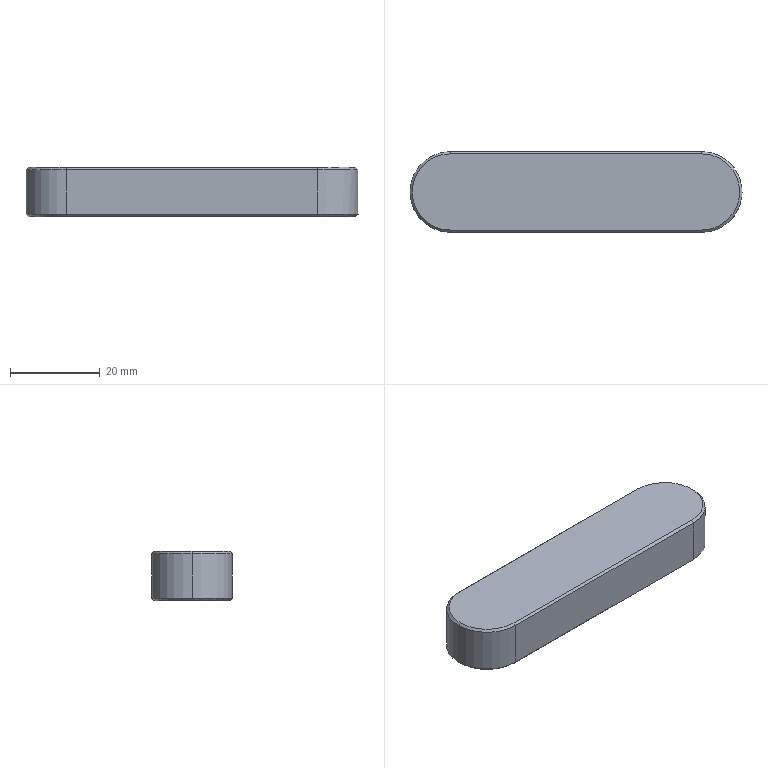Part | SolidWorks | features Chamfer 1, Extrusion 1 | 1 solid | 17 faces | box 74 x 18 x 11 mm | volume 13845 mm3 | plane 8 | cone 6 | cylinder 3 | commonest cylinder face diameters 18 x3
STEP:
#1=CARTESIAN_POINT('',(-36.5,0.,11.));
#2=VERTEX_POINT('',#1);
#3=CARTESIAN_POINT('',(-28.,-8.5,11.));
#4=VERTEX_POINT('',#3);
#5=CARTESIAN_POINT('',(-28.,0.,11.));
#6=DIRECTION('',(0.,0.,1.));
#7=DIRECTION('',(1.,0.,0.));
#8=AXIS2_PLACEMENT_3D('',#5,#6,#7);
#9=CIRCLE('',#8,8.5);
#10=EDGE_CURVE('',#2,#4,#9,.T.);
#11=ORIENTED_EDGE('',*,*,#10,.F.);
#12=CARTESIAN_POINT('',(-37.,0.,10.5));
#13=VERTEX_POINT('',#12);
#14=CARTESIAN_POINT('',(-36.5,0.,11.));
#15=DIRECTION('',(-0.7071,0.,-0.7071));
#16=VECTOR('',#15,1000.);
#17=LINE('',#14,#16);
#18=EDGE_CURVE('',#2,#13,#17,.T.);
#19=ORIENTED_EDGE('',*,*,#18,.T.);
#20=CARTESIAN_POINT('',(-28.,-9.,10.5));
#21=VERTEX_POINT('',#20);
#22=CARTESIAN_POINT('',(-28.,0.,10.5));
#23=DIRECTION('',(0.,0.,-1.));
#24=DIRECTION('',(1.,0.,0.));
#25=AXIS2_PLACEMENT_3D('',#22,#23,#24);
#26=CIRCLE('',#25,9.);
#27=EDGE_CURVE('',#21,#13,#26,.T.);
#28=ORIENTED_EDGE('',*,*,#27,.F.);
#29=CARTESIAN_POINT('',(-28.,-9.,10.5));
#30=DIRECTION('',(0.,0.7071,0.7071));
#31=VECTOR('',#30,1000.);
#32=LINE('',#29,#31);
#33=EDGE_CURVE('',#21,#4,#32,.T.);
#34=ORIENTED_EDGE('',*,*,#33,.T.);
#35=EDGE_LOOP('',(#11,#19,#28,#34));
#36=FACE_OUTER_BOUND('',#35,.T.);
#37=CARTESIAN_POINT('',(-28.,0.,11.));
#38=DIRECTION('',(0.,0.,-1.));
#39=DIRECTION('',(-1.,0.,0.));
#40=AXIS2_PLACEMENT_3D('',#37,#38,#39);
#41=CONICAL_SURFACE('',#40,8.5,0.7854);
#42=ADVANCED_FACE('',(#36),#41,.T.);
#43=CARTESIAN_POINT('',(36.5,0.,0.));
#44=VERTEX_POINT('',#43);
#45=CARTESIAN_POINT('',(28.,-8.5,0.));
#46=VERTEX_POINT('',#45);
#47=CARTESIAN_POINT('',(28.,0.,0.));
#48=DIRECTION('',(0.,0.,-1.));
#49=DIRECTION('',(1.,0.,0.));
#50=AXIS2_PLACEMENT_3D('',#47,#48,#49);
#51=CIRCLE('',#50,8.5);
#52=EDGE_CURVE('',#44,#46,#51,.T.);
#53=ORIENTED_EDGE('',*,*,#52,.F.);
#54=CARTESIAN_POINT('',(37.,0.,0.5));
#55=VERTEX_POINT('',#54);
#56=CARTESIAN_POINT('',(37.,0.,0.5));
#57=DIRECTION('',(0.7071,0.,0.7071));
#58=VECTOR('',#57,1000.);
#59=LINE('',#56,#58);
#60=EDGE_CURVE('',#44,#55,#59,.T.);
#61=ORIENTED_EDGE('',*,*,#60,.T.);
#62=CARTESIAN_POINT('',(28.,-9.,0.5));
#63=VERTEX_POINT('',#62);
#64=CARTESIAN_POINT('',(28.,0.,0.5));
#65=DIRECTION('',(0.,0.,1.));
#66=DIRECTION('',(1.,0.,0.));
#67=AXIS2_PLACEMENT_3D('',#64,#65,#66);
#68=CIRCLE('',#67,9.);
#69=EDGE_CURVE('',#63,#55,#68,.T.);
#70=ORIENTED_EDGE('',*,*,#69,.F.);
#71=CARTESIAN_POINT('',(28.,-8.5,0.));
#72=DIRECTION('',(0.,-0.7071,0.7071));
#73=VECTOR('',#72,1000.);
#74=LINE('',#71,#73);
#75=EDGE_CURVE('',#46,#63,#74,.T.);
#76=ORIENTED_EDGE('',*,*,#75,.F.);
#77=EDGE_LOOP('',(#53,#61,#70,#76));
#78=FACE_OUTER_BOUND('',#77,.T.);
#79=CARTESIAN_POINT('',(28.,0.,0.5));
#80=DIRECTION('',(0.,0.,1.));
#81=DIRECTION('',(1.,0.,0.));
#82=AXIS2_PLACEMENT_3D('',#79,#80,#81);
#83=CONICAL_SURFACE('',#82,9.,0.7854);
#84=ADVANCED_FACE('',(#78),#83,.T.);
#85=ORIENTED_EDGE('',*,*,#27,.T.);
#86=CARTESIAN_POINT('',(-37.,0.,0.5));
#87=VERTEX_POINT('',#86);
#88=CARTESIAN_POINT('',(-37.,0.,11.));
#89=DIRECTION('',(0.,0.,-1.));
#90=VECTOR('',#89,1000.);
#91=LINE('',#88,#90);
#92=EDGE_CURVE('',#13,#87,#91,.T.);
#93=ORIENTED_EDGE('',*,*,#92,.T.);
#94=CARTESIAN_POINT('',(-28.,-9.,0.5));
#95=VERTEX_POINT('',#94);
#96=CARTESIAN_POINT('',(-28.,0.,0.5));
#97=DIRECTION('',(0.,0.,1.));
#98=DIRECTION('',(1.,0.,0.));
#99=AXIS2_PLACEMENT_3D('',#96,#97,#98);
#100=CIRCLE('',#99,9.);
#101=EDGE_CURVE('',#87,#95,#100,.T.);
#102=ORIENTED_EDGE('',*,*,#101,.T.);
#103=CARTESIAN_POINT('',(-28.,-9.,11.));
#104=DIRECTION('',(0.,0.,-1.));
#105=VECTOR('',#104,1000.);
#106=LINE('',#103,#105);
#107=EDGE_CURVE('',#21,#95,#106,.T.);
#108=ORIENTED_EDGE('',*,*,#107,.F.);
#109=EDGE_LOOP('',(#85,#93,#102,#108));
#110=FACE_OUTER_BOUND('',#109,.T.);
#111=CARTESIAN_POINT('',(-28.,0.,11.));
#112=DIRECTION('',(0.,0.,-1.));
#113=DIRECTION('',(-1.,0.,0.));
#114=AXIS2_PLACEMENT_3D('',#111,#112,#113);
#115=CYLINDRICAL_SURFACE('',#114,9.);
#116=ADVANCED_FACE('',(#110),#115,.T.);
#117=ORIENTED_EDGE('',*,*,#92,.F.);
#118=CARTESIAN_POINT('',(-28.,9.,10.5));
#119=VERTEX_POINT('',#118);
#120=CARTESIAN_POINT('',(-28.,0.,10.5));
#121=DIRECTION('',(0.,0.,-1.));
#122=DIRECTION('',(1.,0.,0.));
#123=AXIS2_PLACEMENT_3D('',#120,#121,#122);
#124=CIRCLE('',#123,9.);
#125=EDGE_CURVE('',#13,#119,#124,.T.);
#126=ORIENTED_EDGE('',*,*,#125,.T.);
#127=CARTESIAN_POINT('',(-28.,9.,0.5));
#128=VERTEX_POINT('',#127);
#129=CARTESIAN_POINT('',(-28.,9.,11.));
#130=DIRECTION('',(0.,0.,-1.));
#131=VECTOR('',#130,1000.);
#132=LINE('',#129,#131);
#133=EDGE_CURVE('',#119,#128,#132,.T.);
#134=ORIENTED_EDGE('',*,*,#133,.T.);
#135=CARTESIAN_POINT('',(-28.,0.,0.5));
#136=DIRECTION('',(0.,0.,1.));
#137=DIRECTION('',(1.,0.,0.));
#138=AXIS2_PLACEMENT_3D('',#135,#136,#137);
#139=CIRCLE('',#138,9.);
#140=EDGE_CURVE('',#128,#87,#139,.T.);
#141=ORIENTED_EDGE('',*,*,#140,.T.);
#142=EDGE_LOOP('',(#117,#126,#134,#141));
#143=FACE_OUTER_BOUND('',#142,.T.);
#144=CARTESIAN_POINT('',(-28.,0.,11.));
#145=DIRECTION('',(0.,0.,-1.));
#146=DIRECTION('',(-1.,0.,0.));
#147=AXIS2_PLACEMENT_3D('',#144,#145,#146);
#148=CYLINDRICAL_SURFACE('',#147,9.);
#149=ADVANCED_FACE('',(#143),#148,.T.);
#150=ORIENTED_EDGE('',*,*,#107,.T.);
#151=CARTESIAN_POINT('',(0.,-9.,0.5));
#152=DIRECTION('',(1.,0.,0.));
#153=VECTOR('',#152,1000.);
#154=LINE('',#151,#153);
#155=EDGE_CURVE('',#95,#63,#154,.T.);
#156=ORIENTED_EDGE('',*,*,#155,.T.);
#157=CARTESIAN_POINT('',(28.,-9.,10.5));
#158=VERTEX_POINT('',#157);
#159=CARTESIAN_POINT('',(28.,-9.,11.));
#160=DIRECTION('',(0.,0.,-1.));
#161=VECTOR('',#160,1000.);
#162=LINE('',#159,#161);
#163=EDGE_CURVE('',#158,#63,#162,.T.);
#164=ORIENTED_EDGE('',*,*,#163,.F.);
#165=CARTESIAN_POINT('',(-28.,-9.,10.5));
#166=DIRECTION('',(-1.,0.,0.));
#167=VECTOR('',#166,1000.);
#168=LINE('',#165,#167);
#169=EDGE_CURVE('',#158,#21,#168,.T.);
#170=ORIENTED_EDGE('',*,*,#169,.T.);
#171=EDGE_LOOP('',(#150,#156,#164,#170));
#172=FACE_OUTER_BOUND('',#171,.T.);
#173=CARTESIAN_POINT('',(0.,-9.,11.));
#174=DIRECTION('',(0.,1.,0.));
#175=DIRECTION('',(0.,0.,1.));
#176=AXIS2_PLACEMENT_3D('',#173,#174,#175);
#177=PLANE('',#176);
#178=ADVANCED_FACE('',(#172),#177,.F.);
#179=ORIENTED_EDGE('',*,*,#163,.T.);
#180=ORIENTED_EDGE('',*,*,#69,.T.);
#181=CARTESIAN_POINT('',(28.,9.,0.5));
#182=VERTEX_POINT('',#181);
#183=CARTESIAN_POINT('',(28.,0.,0.5));
#184=DIRECTION('',(0.,0.,1.));
#185=DIRECTION('',(1.,0.,0.));
#186=AXIS2_PLACEMENT_3D('',#183,#184,#185);
#187=CIRCLE('',#186,9.);
#188=EDGE_CURVE('',#55,#182,#187,.T.);
#189=ORIENTED_EDGE('',*,*,#188,.T.);
#190=CARTESIAN_POINT('',(28.,9.,10.5));
#191=VERTEX_POINT('',#190);
#192=CARTESIAN_POINT('',(28.,9.,11.));
#193=DIRECTION('',(0.,0.,-1.));
#194=VECTOR('',#193,1000.);
#195=LINE('',#192,#194);
#196=EDGE_CURVE('',#191,#182,#195,.T.);
#197=ORIENTED_EDGE('',*,*,#196,.F.);
#198=CARTESIAN_POINT('',(28.,0.,10.5));
#199=DIRECTION('',(0.,0.,-1.));
#200=DIRECTION('',(1.,0.,0.));
#201=AXIS2_PLACEMENT_3D('',#198,#199,#200);
#202=CIRCLE('',#201,9.);
#203=EDGE_CURVE('',#191,#158,#202,.T.);
#204=ORIENTED_EDGE('',*,*,#203,.T.);
#205=EDGE_LOOP('',(#179,#180,#189,#197,#204));
#206=FACE_OUTER_BOUND('',#205,.T.);
#207=CARTESIAN_POINT('',(28.,0.,11.));
#208=DIRECTION('',(0.,0.,-1.));
#209=DIRECTION('',(-1.,0.,0.));
#210=AXIS2_PLACEMENT_3D('',#207,#208,#209);
#211=CYLINDRICAL_SURFACE('',#210,9.);
#212=ADVANCED_FACE('',(#206),#211,.T.);
#213=ORIENTED_EDGE('',*,*,#196,.T.);
#214=CARTESIAN_POINT('',(0.,9.,0.5));
#215=DIRECTION('',(-1.,0.,0.));
#216=VECTOR('',#215,1000.);
#217=LINE('',#214,#216);
#218=EDGE_CURVE('',#182,#128,#217,.T.);
#219=ORIENTED_EDGE('',*,*,#218,.T.);
#220=ORIENTED_EDGE('',*,*,#133,.F.);
#221=CARTESIAN_POINT('',(28.,9.,10.5));
#222=DIRECTION('',(1.,0.,0.));
#223=VECTOR('',#222,1000.);
#224=LINE('',#221,#223);
#225=EDGE_CURVE('',#119,#191,#224,.T.);
#226=ORIENTED_EDGE('',*,*,#225,.T.);
#227=EDGE_LOOP('',(#213,#219,#220,#226));
#228=FACE_OUTER_BOUND('',#227,.T.);
#229=CARTESIAN_POINT('',(0.,9.,11.));
#230=DIRECTION('',(0.,-1.,0.));
#231=DIRECTION('',(0.,0.,-1.));
#232=AXIS2_PLACEMENT_3D('',#229,#230,#231);
#233=PLANE('',#232);
#234=ADVANCED_FACE('',(#228),#233,.F.);
#235=CARTESIAN_POINT('',(28.,8.5,11.));
#236=VERTEX_POINT('',#235);
#237=CARTESIAN_POINT('',(-28.,8.5,11.));
#238=VERTEX_POINT('',#237);
#239=CARTESIAN_POINT('',(-28.,8.5,11.));
#240=DIRECTION('',(-1.,0.,0.));
#241=VECTOR('',#240,1000.);
#242=LINE('',#239,#241);
#243=EDGE_CURVE('',#236,#238,#242,.T.);
#244=ORIENTED_EDGE('',*,*,#243,.T.);
#245=CARTESIAN_POINT('',(-28.,0.,11.));
#246=DIRECTION('',(0.,0.,1.));
#247=DIRECTION('',(1.,0.,0.));
#248=AXIS2_PLACEMENT_3D('',#245,#246,#247);
#249=CIRCLE('',#248,8.5);
#250=EDGE_CURVE('',#238,#2,#249,.T.);
#251=ORIENTED_EDGE('',*,*,#250,.T.);
#252=ORIENTED_EDGE('',*,*,#10,.T.);
#253=CARTESIAN_POINT('',(28.,-8.5,11.));
#254=VERTEX_POINT('',#253);
#255=CARTESIAN_POINT('',(28.,-8.5,11.));
#256=DIRECTION('',(1.,0.,0.));
#257=VECTOR('',#256,1000.);
#258=LINE('',#255,#257);
#259=EDGE_CURVE('',#4,#254,#258,.T.);
#260=ORIENTED_EDGE('',*,*,#259,.T.);
#261=CARTESIAN_POINT('',(28.,0.,11.));
#262=DIRECTION('',(0.,0.,1.));
#263=DIRECTION('',(1.,0.,0.));
#264=AXIS2_PLACEMENT_3D('',#261,#262,#263);
#265=CIRCLE('',#264,8.5);
#266=EDGE_CURVE('',#254,#236,#265,.T.);
#267=ORIENTED_EDGE('',*,*,#266,.T.);
#268=EDGE_LOOP('',(#244,#251,#252,#260,#267));
#269=FACE_OUTER_BOUND('',#268,.T.);
#270=CARTESIAN_POINT('',(-28.,0.,11.));
#271=DIRECTION('',(0.,0.,1.));
#272=DIRECTION('',(1.,0.,0.));
#273=AXIS2_PLACEMENT_3D('',#270,#271,#272);
#274=PLANE('',#273);
#275=ADVANCED_FACE('',(#269),#274,.T.);
#276=CARTESIAN_POINT('',(28.,8.5,0.));
#277=VERTEX_POINT('',#276);
#278=CARTESIAN_POINT('',(28.,0.,0.));
#279=DIRECTION('',(0.,0.,-1.));
#280=DIRECTION('',(1.,0.,0.));
#281=AXIS2_PLACEMENT_3D('',#278,#279,#280);
#282=CIRCLE('',#281,8.5);
#283=EDGE_CURVE('',#277,#44,#282,.T.);
#284=ORIENTED_EDGE('',*,*,#283,.T.);
#285=ORIENTED_EDGE('',*,*,#52,.T.);
#286=CARTESIAN_POINT('',(-28.,-8.5,0.));
#287=VERTEX_POINT('',#286);
#288=CARTESIAN_POINT('',(-28.,-8.5,0.));
#289=DIRECTION('',(-1.,0.,0.));
#290=VECTOR('',#289,1000.);
#291=LINE('',#288,#290);
#292=EDGE_CURVE('',#46,#287,#291,.T.);
#293=ORIENTED_EDGE('',*,*,#292,.T.);
#294=CARTESIAN_POINT('',(-28.,8.5,0.));
#295=VERTEX_POINT('',#294);
#296=CARTESIAN_POINT('',(-28.,0.,0.));
#297=DIRECTION('',(0.,0.,-1.));
#298=DIRECTION('',(1.,0.,0.));
#299=AXIS2_PLACEMENT_3D('',#296,#297,#298);
#300=CIRCLE('',#299,8.5);
#301=EDGE_CURVE('',#287,#295,#300,.T.);
#302=ORIENTED_EDGE('',*,*,#301,.T.);
#303=CARTESIAN_POINT('',(-28.,8.5,0.));
#304=DIRECTION('',(1.,0.,0.));
#305=VECTOR('',#304,1000.);
#306=LINE('',#303,#305);
#307=EDGE_CURVE('',#295,#277,#306,.T.);
#308=ORIENTED_EDGE('',*,*,#307,.T.);
#309=EDGE_LOOP('',(#284,#285,#293,#302,#308));
#310=FACE_OUTER_BOUND('',#309,.T.);
#311=CARTESIAN_POINT('',(-28.,0.,0.));
#312=DIRECTION('',(0.,0.,1.));
#313=DIRECTION('',(1.,0.,0.));
#314=AXIS2_PLACEMENT_3D('',#311,#312,#313);
#315=PLANE('',#314);
#316=ADVANCED_FACE('',(#310),#315,.F.);
#317=CARTESIAN_POINT('',(28.,8.5,0.));
#318=DIRECTION('',(0.,0.7071,0.7071));
#319=VECTOR('',#318,1000.);
#320=LINE('',#317,#319);
#321=EDGE_CURVE('',#277,#182,#320,.T.);
#322=ORIENTED_EDGE('',*,*,#321,.F.);
#323=ORIENTED_EDGE('',*,*,#307,.F.);
#324=CARTESIAN_POINT('',(-28.,9.,0.5));
#325=DIRECTION('',(0.,-0.7071,-0.7071));
#326=VECTOR('',#325,1000.);
#327=LINE('',#324,#326);
#328=EDGE_CURVE('',#128,#295,#327,.T.);
#329=ORIENTED_EDGE('',*,*,#328,.F.);
#330=ORIENTED_EDGE('',*,*,#218,.F.);
#331=EDGE_LOOP('',(#322,#323,#329,#330));
#332=FACE_OUTER_BOUND('',#331,.T.);
#333=CARTESIAN_POINT('',(0.,9.,0.5));
#334=DIRECTION('',(0.,-0.7071,0.7071));
#335=DIRECTION('',(-1.,0.,0.));
#336=AXIS2_PLACEMENT_3D('',#333,#334,#335);
#337=PLANE('',#336);
#338=ADVANCED_FACE('',(#332),#337,.F.);
#339=ORIENTED_EDGE('',*,*,#328,.T.);
#340=ORIENTED_EDGE('',*,*,#301,.F.);
#341=CARTESIAN_POINT('',(-28.,-9.,0.5));
#342=DIRECTION('',(0.,0.7071,-0.7071));
#343=VECTOR('',#342,1000.);
#344=LINE('',#341,#343);
#345=EDGE_CURVE('',#95,#287,#344,.T.);
#346=ORIENTED_EDGE('',*,*,#345,.F.);
#347=ORIENTED_EDGE('',*,*,#101,.F.);
#348=ORIENTED_EDGE('',*,*,#140,.F.);
#349=EDGE_LOOP('',(#339,#340,#346,#347,#348));
#350=FACE_OUTER_BOUND('',#349,.T.);
#351=CARTESIAN_POINT('',(-28.,0.,0.5));
#352=DIRECTION('',(0.,0.,1.));
#353=DIRECTION('',(1.,0.,0.));
#354=AXIS2_PLACEMENT_3D('',#351,#352,#353);
#355=CONICAL_SURFACE('',#354,9.,0.7854);
#356=ADVANCED_FACE('',(#350),#355,.T.);
#357=ORIENTED_EDGE('',*,*,#60,.F.);
#358=ORIENTED_EDGE('',*,*,#283,.F.);
#359=ORIENTED_EDGE('',*,*,#321,.T.);
#360=ORIENTED_EDGE('',*,*,#188,.F.);
#361=EDGE_LOOP('',(#357,#358,#359,#360));
#362=FACE_OUTER_BOUND('',#361,.T.);
#363=CARTESIAN_POINT('',(28.,0.,0.5));
#364=DIRECTION('',(0.,0.,1.));
#365=DIRECTION('',(1.,0.,0.));
#366=AXIS2_PLACEMENT_3D('',#363,#364,#365);
#367=CONICAL_SURFACE('',#366,9.,0.7854);
#368=ADVANCED_FACE('',(#362),#367,.T.);
#369=ORIENTED_EDGE('',*,*,#345,.T.);
#370=ORIENTED_EDGE('',*,*,#292,.F.);
#371=ORIENTED_EDGE('',*,*,#75,.T.);
#372=ORIENTED_EDGE('',*,*,#155,.F.);
#373=EDGE_LOOP('',(#369,#370,#371,#372));
#374=FACE_OUTER_BOUND('',#373,.T.);
#375=CARTESIAN_POINT('',(0.,-9.,0.5));
#376=DIRECTION('',(0.,0.7071,0.7071));
#377=DIRECTION('',(1.,0.,0.));
#378=AXIS2_PLACEMENT_3D('',#375,#376,#377);
#379=PLANE('',#378);
#380=ADVANCED_FACE('',(#374),#379,.F.);
#381=CARTESIAN_POINT('',(28.,-9.,10.5));
#382=DIRECTION('',(0.,0.7071,0.7071));
#383=VECTOR('',#382,1000.);
#384=LINE('',#381,#383);
#385=EDGE_CURVE('',#158,#254,#384,.T.);
#386=ORIENTED_EDGE('',*,*,#385,.F.);
#387=ORIENTED_EDGE('',*,*,#203,.F.);
#388=CARTESIAN_POINT('',(28.,8.5,11.));
#389=DIRECTION('',(0.,0.7071,-0.7071));
#390=VECTOR('',#389,1000.);
#391=LINE('',#388,#390);
#392=EDGE_CURVE('',#236,#191,#391,.T.);
#393=ORIENTED_EDGE('',*,*,#392,.F.);
#394=ORIENTED_EDGE('',*,*,#266,.F.);
#395=EDGE_LOOP('',(#386,#387,#393,#394));
#396=FACE_OUTER_BOUND('',#395,.T.);
#397=CARTESIAN_POINT('',(28.,0.,11.));
#398=DIRECTION('',(0.,0.,-1.));
#399=DIRECTION('',(-1.,0.,0.));
#400=AXIS2_PLACEMENT_3D('',#397,#398,#399);
#401=CONICAL_SURFACE('',#400,8.5,0.7854);
#402=ADVANCED_FACE('',(#396),#401,.T.);
#403=ORIENTED_EDGE('',*,*,#392,.T.);
#404=ORIENTED_EDGE('',*,*,#225,.F.);
#405=CARTESIAN_POINT('',(-28.,8.5,11.));
#406=DIRECTION('',(0.,0.7071,-0.7071));
#407=VECTOR('',#406,1000.);
#408=LINE('',#405,#407);
#409=EDGE_CURVE('',#238,#119,#408,.T.);
#410=ORIENTED_EDGE('',*,*,#409,.F.);
#411=ORIENTED_EDGE('',*,*,#243,.F.);
#412=EDGE_LOOP('',(#403,#404,#410,#411));
#413=FACE_OUTER_BOUND('',#412,.T.);
#414=CARTESIAN_POINT('',(-28.,8.5,11.));
#415=DIRECTION('',(0.,0.7071,0.7071));
#416=DIRECTION('',(1.,0.,0.));
#417=AXIS2_PLACEMENT_3D('',#414,#415,#416);
#418=PLANE('',#417);
#419=ADVANCED_FACE('',(#413),#418,.T.);
#420=ORIENTED_EDGE('',*,*,#385,.T.);
#421=ORIENTED_EDGE('',*,*,#259,.F.);
#422=ORIENTED_EDGE('',*,*,#33,.F.);
#423=ORIENTED_EDGE('',*,*,#169,.F.);
#424=EDGE_LOOP('',(#420,#421,#422,#423));
#425=FACE_OUTER_BOUND('',#424,.T.);
#426=CARTESIAN_POINT('',(-28.,-8.5,11.));
#427=DIRECTION('',(0.,-0.7071,0.7071));
#428=DIRECTION('',(-1.,0.,0.));
#429=AXIS2_PLACEMENT_3D('',#426,#427,#428);
#430=PLANE('',#429);
#431=ADVANCED_FACE('',(#425),#430,.T.);
#432=ORIENTED_EDGE('',*,*,#18,.F.);
#433=ORIENTED_EDGE('',*,*,#250,.F.);
#434=ORIENTED_EDGE('',*,*,#409,.T.);
#435=ORIENTED_EDGE('',*,*,#125,.F.);
#436=EDGE_LOOP('',(#432,#433,#434,#435));
#437=FACE_OUTER_BOUND('',#436,.T.);
#438=CARTESIAN_POINT('',(-28.,0.,11.));
#439=DIRECTION('',(0.,0.,-1.));
#440=DIRECTION('',(-1.,0.,0.));
#441=AXIS2_PLACEMENT_3D('',#438,#439,#440);
#442=CONICAL_SURFACE('',#441,8.5,0.7854);
#443=ADVANCED_FACE('',(#437),#442,.T.);
#444=CLOSED_SHELL('',(#42,#84,#116,#149,#178,#212,#234,#275,#316,#338,#356,#368,#380,#402,#419,#431,#443));
#445=MANIFOLD_SOLID_BREP('',#444);
#446=CARTESIAN_POINT('',(0.,0.,0.));
#447=DIRECTION('',(0.,0.,1.));
#448=DIRECTION('',(1.,0.,0.));
#449=AXIS2_PLACEMENT_3D('',#446,#447,#448);
#450=(LENGTH_UNIT()NAMED_UNIT(*)SI_UNIT(.MILLI.,.METRE.));
#451=UNCERTAINTY_MEASURE_WITH_UNIT(LENGTH_MEASURE(0.00001),#450,'','');
#452=(NAMED_UNIT(*)PLANE_ANGLE_UNIT()SI_UNIT($,.RADIAN.));
#453=(NAMED_UNIT(*)SI_UNIT($,.STERADIAN.)SOLID_ANGLE_UNIT());
#454=(GEOMETRIC_REPRESENTATION_CONTEXT(3)GLOBAL_UNCERTAINTY_ASSIGNED_CONTEXT((#451))GLOBAL_UNIT_ASSIGNED_CONTEXT((#450,#452,#453))REPRESENTATION_CONTEXT('',''));
#455=ADVANCED_BREP_SHAPE_REPRESENTATION('',(#445,#449),#454);